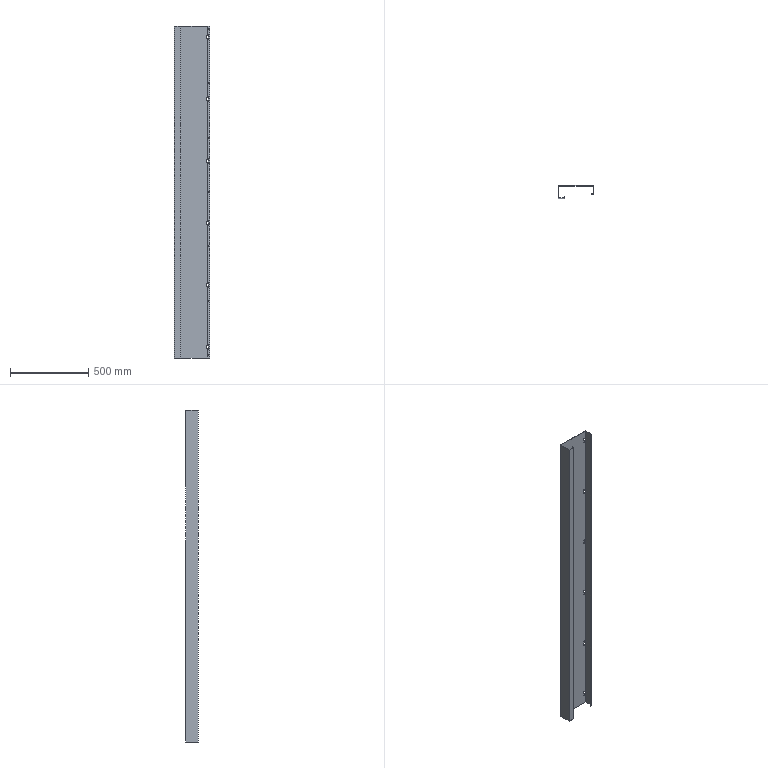Part | SolidWorks | features ICE 6, Cut 4, EdgeFlange 2, MirrorPattern 2, Fillet 1, FlatPattern 1, SMBaseFlange 1, SheetMetal 1 | 1 solid | 128 faces | box 225 x 80 x 2116 mm | volume 1054460 mm3 | plane 72 | cylinder 56 | commonest cylinder face diameters 6.2 x28 9 x18 1 x5 3.4 x5